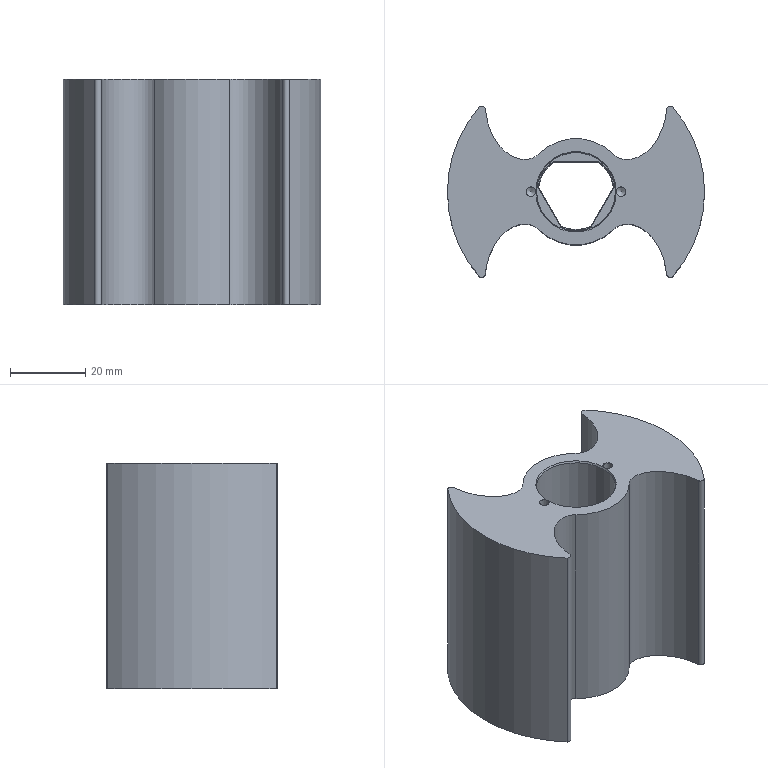NC program | NX | posted with a generic post | part box 68.489 x 45.577 x 60 mm
Lines 4138 to 5071 of 7016:
(CUTTERCOMP12 , TOOL : D12)
N8274 T12 M6
N8276 G54
N8278 G17 G0 G90 X33.59 Y-26.428 S5000 M3
N8280 G43 Z30. H12
N8282 Z1.
N8284 G94 G1 Z-1. F1250.
N8286 G41 X33.497 Y-26.392 D12
N8288 X31.512 Y-26.006
N8290 G3 X30.378 Y-26.397 R1.2
N8292 G2 X18.216 Y-22.529 R6.95
N8294 G3 X17.367 Y-18.826 R14.157
N8296 X16.037 Y-16.381 R9.956
N8298 X14.862 Y-15.174 R6.285
N8300 X13.864 Y-14.63 R3.173
N8302 G2 X-13.864 Y-14.629 R20.155
N8304 G3 X-14.862 Y-15.174 R3.211
N8306 X-16.324 Y-16.786 R6.7
N8308 X-17.543 Y-19.315 R10.577
N8310 X-18.216 Y-22.527 R14.318
N8312 G2 X-30.378 Y-26.397 R6.95
N8314 G3 X-31.512 Y-26.006 R1.2
N8316 G1 X-33.497 Y-26.392
N8318 G40
N8320 X-33.59 Y-26.428
N8322 Z1.
N8324 G0 X33.59 Z0.
N8326 G1 Z-2.
N8328 G41 X33.497 Y-26.392
N8330 X31.512 Y-26.006
N8332 G3 X30.378 Y-26.397 R1.2
N8334 G2 X18.216 Y-22.529 R6.95
N8336 G3 X17.367 Y-18.826 R14.159
N8338 X16.037 Y-16.381 R9.956
N8340 X14.862 Y-15.174 R6.285
N8342 X13.864 Y-14.63 R3.174
N8344 G2 X-13.864 Y-14.629 R20.155
N8346 G3 X-14.862 Y-15.174 R3.213
N8348 X-16.324 Y-16.786 R6.7
N8350 X-17.543 Y-19.315 R10.578
N8352 X-18.216 Y-22.527 R14.323
N8354 G2 X-30.378 Y-26.397 R6.95
N8356 G3 X-31.512 Y-26.006 R1.2
N8358 G1 X-33.497 Y-26.392
N8360 G40
N8362 X-33.59 Y-26.428
N8364 Z0.
N8366 G0 Z30.
N8368 X33.59
N8370 Z-1.
N8372 G1 Z-3.
N8374 G41 X33.497 Y-26.392
N8376 X31.512 Y-26.006
N8378 G3 X30.378 Y-26.397 R1.2
N8380 G2 X18.216 Y-22.529 R6.95
N8382 G3 X17.367 Y-18.826 R14.16
N8384 X16.037 Y-16.381 R9.955
N8386 X14.862 Y-15.174 R6.285
N8388 X13.864 Y-14.63 R3.175
N8390 G2 X-13.864 Y-14.629 R20.155
N8392 G3 X-14.862 Y-15.174 R3.214
N8394 X-16.324 Y-16.786 R6.7
N8396 X-17.543 Y-19.315 R10.579
N8398 X-18.216 Y-22.527 R14.328
N8400 G2 X-30.378 Y-26.397 R6.95
N8402 G3 X-31.512 Y-26.006 R1.2
N8404 G1 X-33.497 Y-26.392
N8406 G40
N8408 X-33.59 Y-26.428
N8410 Z-1.
N8412 G0 Z30.
N8414 X33.59
N8416 Z-2.
N8418 G1 Z-4.
N8420 G41 X33.497 Y-26.392
N8422 X31.512 Y-26.006
N8424 G3 X30.378 Y-26.397 R1.2
N8426 G2 X18.216 Y-22.529 R6.95
N8428 G3 X17.367 Y-18.826 R14.162
N8430 X16.037 Y-16.381 R9.955
N8432 X14.862 Y-15.174 R6.285
N8434 X13.864 Y-14.63 R3.175
N8436 G2 X-13.864 Y-14.629 R20.155
N8438 G3 X-14.862 Y-15.174 R3.215
N8440 X-16.039 Y-16.381 R6.439
N8442 X-17.367 Y-18.826 R10.062
N8444 X-18.216 Y-22.527 R14.147
N8446 G2 X-30.378 Y-26.397 R6.95
N8448 G3 X-31.512 Y-26.006 R1.2
N8450 G1 X-33.497 Y-26.392
N8452 G40
N8454 X-33.59 Y-26.428
N8456 Z-2.
N8458 G0 Z30.
N8460 X33.59
N8462 Z-3.
N8464 G1 Z-5.
N8466 G41 X33.497 Y-26.392
N8468 X31.512 Y-26.006
N8470 G3 X30.378 Y-26.397 R1.2
N8472 G2 X18.216 Y-22.529 R6.95
N8474 G3 X17.367 Y-18.826 R14.164
N8476 X16.037 Y-16.381 R9.955
N8478 X14.862 Y-15.174 R6.284
N8480 X13.864 Y-14.63 R3.176
N8482 G2 X-13.864 Y-14.629 R20.155
N8484 G3 X-14.862 Y-15.174 R3.216
N8486 X-16.039 Y-16.381 R6.438
N8488 X-17.367 Y-18.826 R10.06
N8490 X-18.216 Y-22.527 R14.13
N8492 G2 X-30.378 Y-26.397 R6.95
N8494 G3 X-31.512 Y-26.006 R1.2
N8496 G1 X-33.497 Y-26.392
N8498 G40
N8500 X-33.59 Y-26.428
N8502 Z-3.
N8504 G0 Z30.
N8506 X33.59
N8508 Z-4.
N8510 G1 Z-6.
N8512 G41 X33.497 Y-26.392
N8514 X31.512 Y-26.006
N8516 G3 X30.378 Y-26.397 R1.2
N8518 G2 X18.216 Y-22.529 R6.95
N8520 G3 X17.367 Y-18.826 R14.165
N8522 X16.037 Y-16.381 R9.954
N8524 X14.862 Y-15.174 R6.284
N8526 X13.864 Y-14.63 R3.177
N8528 G2 X-13.864 Y-14.629 R20.155
N8530 G3 X-14.862 Y-15.174 R3.217
N8532 X-16.039 Y-16.381 R6.436
N8534 X-17.367 Y-18.826 R10.058
N8536 X-18.216 Y-22.527 R14.133
N8538 G2 X-30.378 Y-26.397 R6.95
N8540 G3 X-31.512 Y-26.006 R1.2
N8542 G1 X-33.497 Y-26.392
N8544 G40
N8546 X-33.59 Y-26.428
N8548 Z-4.
N8550 G0 Z30.
N8552 X33.59
N8554 Z-5.
N8556 G1 Z-7.
N8558 G41 X33.497 Y-26.392
N8560 X31.512 Y-26.006
N8562 G3 X30.378 Y-26.397 R1.2
N8564 G2 X18.216 Y-22.529 R6.95
N8566 G3 X17.367 Y-18.826 R14.167
N8568 X16.037 Y-16.381 R9.954
N8570 X14.862 Y-15.174 R6.284
N8572 X13.864 Y-14.63 R3.177
N8574 G2 X-13.864 Y-14.629 R20.155
N8576 G3 X-14.862 Y-15.174 R3.218
N8578 X-16.039 Y-16.381 R6.435
N8580 X-17.367 Y-18.826 R10.057
N8582 X-18.216 Y-22.527 R14.137
N8584 G2 X-30.378 Y-26.397 R6.95
N8586 G3 X-31.512 Y-26.006 R1.2
N8588 G1 X-33.497 Y-26.392
N8590 G40
N8592 X-33.59 Y-26.428
N8594 Z-5.
N8596 G0 Z30.
N8598 X33.59
N8600 Z-6.
N8602 G1 Z-8.
N8604 G41 X33.497 Y-26.392
N8606 X31.512 Y-26.006
N8608 G3 X30.378 Y-26.397 R1.2
N8610 G2 X18.216 Y-22.529 R6.95
N8612 G3 X17.367 Y-18.826 R14.169
N8614 X16.037 Y-16.381 R9.954
N8616 X14.862 Y-15.174 R6.275
N8618 X13.864 Y-14.63 R3.178
N8620 G2 X-13.864 Y-14.629 R20.155
N8622 G3 X-14.862 Y-15.174 R3.219
N8624 X-16.038 Y-16.381 R6.434
N8626 X-17.367 Y-18.826 R10.055
N8628 X-18.216 Y-22.527 R14.141
N8630 G2 X-30.378 Y-26.397 R6.95
N8632 G3 X-31.512 Y-26.006 R1.2
N8634 G1 X-33.497 Y-26.392
N8636 G40
N8638 X-33.59 Y-26.428
N8640 Z-6.
N8642 G0 Z30.
N8644 X33.59
N8646 Z-7.
N8648 G1 Z-9.
N8650 G41 X33.497 Y-26.392
N8652 X31.512 Y-26.006
N8654 G3 X30.378 Y-26.397 R1.2
N8656 G2 X18.216 Y-22.529 R6.95
N8658 G3 X17.367 Y-18.826 R14.17
N8660 X16.037 Y-16.381 R9.953
N8662 X14.862 Y-15.174 R6.275
N8664 X13.864 Y-14.63 R3.179
N8666 G2 X-13.864 Y-14.629 R20.155
N8668 G3 X-14.862 Y-15.174 R3.22
N8670 X-16.038 Y-16.381 R6.433
N8672 X-17.367 Y-18.826 R10.054
N8674 X-18.216 Y-22.527 R14.144
N8676 G2 X-30.378 Y-26.397 R6.95
N8678 G3 X-31.512 Y-26.006 R1.2
N8680 G1 X-33.497 Y-26.392
N8682 G40
N8684 X-33.59 Y-26.428
N8686 Z-7.
N8688 G0 Z30.
N8690 X33.59
N8692 Z-8.
N8694 G1 Z-10.
N8696 G41 X33.497 Y-26.392
N8698 X31.512 Y-26.006
N8700 G3 X30.378 Y-26.397 R1.2
N8702 G2 X18.216 Y-22.529 R6.95
N8704 G3 X17.367 Y-18.826 R14.172
N8706 X16.037 Y-16.381 R9.953
N8708 X14.862 Y-15.174 R6.274
N8710 X13.864 Y-14.63 R3.179
N8712 G2 X-13.864 Y-14.629 R20.155
N8714 G3 X-14.862 Y-15.174 R3.221
N8716 X-16.038 Y-16.381 R6.432
N8718 X-17.367 Y-18.826 R10.052
N8720 X-18.216 Y-22.527 R14.148
N8722 G2 X-30.378 Y-26.397 R6.95
N8724 G3 X-31.512 Y-26.006 R1.2
N8726 G1 X-33.497 Y-26.392
N8728 G40
N8730 X-33.59 Y-26.428
N8732 Z-8.
N8734 G0 Z30.
N8736 X33.59
N8738 Z-9.
N8740 G1 Z-11.
N8742 G41 X33.497 Y-26.392
N8744 X31.512 Y-26.006
N8746 G3 X30.378 Y-26.397 R1.2
N8748 G2 X18.216 Y-22.529 R6.95
N8750 G3 X17.367 Y-18.826 R14.174
N8752 X16.037 Y-16.381 R9.953
N8754 X14.862 Y-15.174 R6.274
N8756 X13.864 Y-14.63 R3.18
N8758 G2 X-13.864 Y-14.629 R20.155
N8760 G3 X-14.862 Y-15.174 R3.222
N8762 X-16.038 Y-16.381 R6.43
N8764 X-17.367 Y-18.826 R10.051
N8766 X-18.216 Y-22.527 R14.152
N8768 G2 X-30.378 Y-26.397 R6.95
N8770 G3 X-31.512 Y-26.006 R1.2
N8772 G1 X-33.497 Y-26.392
N8774 G40
N8776 X-33.59 Y-26.428
N8778 Z-9.
N8780 G0 Z30.
N8782 X33.59
N8784 Z-10.
N8786 G1 Z-12.
N8788 G41 X33.497 Y-26.392
N8790 X31.512 Y-26.006
N8792 G3 X30.378 Y-26.397 R1.2
N8794 G2 X18.216 Y-22.529 R6.95
N8796 G3 X17.367 Y-18.826 R14.175
N8798 X16.037 Y-16.381 R9.953
N8800 X14.862 Y-15.174 R6.274
N8802 X13.864 Y-14.63 R3.18
N8804 G2 X-13.864 Y-14.629 R20.155
N8806 G3 X-14.862 Y-15.174 R3.223
N8808 X-16.038 Y-16.381 R6.429
N8810 X-17.367 Y-18.826 R10.049
N8812 X-18.216 Y-22.527 R14.155
N8814 G2 X-30.378 Y-26.397 R6.95
N8816 G3 X-31.512 Y-26.006 R1.2
N8818 G1 X-33.497 Y-26.392
N8820 G40
N8822 X-33.59 Y-26.428
N8824 Z-10.
N8826 G0 Z30.
N8828 X33.59
N8830 Z-11.
N8832 G1 Z-13.
N8834 G41 X33.497 Y-26.392
N8836 X31.512 Y-26.006
N8838 G3 X30.378 Y-26.397 R1.2
N8840 G2 X18.216 Y-22.529 R6.95
N8842 G3 X17.367 Y-18.826 R14.177
N8844 X16.037 Y-16.381 R9.952
N8846 X14.862 Y-15.174 R6.274
N8848 X13.864 Y-14.63 R3.181
N8850 G2 X-13.864 Y-14.629 R20.155
N8852 G3 X-14.862 Y-15.174 R3.224
N8854 X-16.038 Y-16.381 R6.428
N8856 X-17.367 Y-18.826 R10.048
N8858 X-18.216 Y-22.527 R14.159
N8860 G2 X-30.378 Y-26.397 R6.95
N8862 G3 X-31.512 Y-26.006 R1.2
N8864 G1 X-33.497 Y-26.392
N8866 G40
N8868 X-33.59 Y-26.428
N8870 Z-11.
N8872 G0 Z30.
N8874 X33.59
N8876 Z-12.
N8878 G1 Z-14.
N8880 G41 X33.497 Y-26.392
N8882 X31.512 Y-26.006
N8884 G3 X30.378 Y-26.397 R1.2
N8886 G2 X18.216 Y-22.529 R6.95
N8888 G3 X17.367 Y-18.826 R14.179
N8890 X16.037 Y-16.381 R9.952
N8892 X14.862 Y-15.174 R6.274
N8894 X13.864 Y-14.63 R3.182
N8896 G2 X-13.864 Y-14.629 R20.155
N8898 G3 X-14.862 Y-15.174 R3.226
N8900 X-16.038 Y-16.381 R6.427
N8902 X-17.367 Y-18.826 R10.046
N8904 X-18.216 Y-22.527 R14.163
N8906 G2 X-30.378 Y-26.397 R6.95
N8908 G3 X-31.512 Y-26.006 R1.2
N8910 G1 X-33.497 Y-26.392
N8912 G40
N8914 X-33.59 Y-26.428
N8916 Z-12.
N8918 G0 Z30.
N8920 X33.59
N8922 Z-13.
N8924 G1 Z-15.
N8926 G41 X33.497 Y-26.392
N8928 X31.512 Y-26.006
N8930 G3 X30.378 Y-26.397 R1.2
N8932 G2 X18.216 Y-22.529 R6.95
N8934 G3 X17.367 Y-18.826 R14.18
N8936 X16.037 Y-16.381 R9.952
N8938 X14.862 Y-15.174 R6.274
N8940 X13.864 Y-14.63 R3.182
N8942 G2 X-13.864 Y-14.629 R20.155
N8944 G3 X-14.862 Y-15.174 R3.227
N8946 X-16.038 Y-16.381 R6.426
N8948 X-17.367 Y-18.826 R10.045
N8950 X-18.216 Y-22.527 R14.167
N8952 G2 X-30.378 Y-26.397 R6.95
N8954 G3 X-31.512 Y-26.006 R1.2
N8956 G1 X-33.497 Y-26.392
N8958 G40
N8960 X-33.59 Y-26.428
N8962 Z-13.
N8964 G0 Z30.
N8966 X33.59
N8968 Z-14.
N8970 G1 Z-16.
N8972 G41 X33.497 Y-26.392
N8974 X31.512 Y-26.006
N8976 G3 X30.378 Y-26.397 R1.2
N8978 G2 X18.216 Y-22.529 R6.95
N8980 G3 X17.367 Y-18.826 R14.182
N8982 X16.037 Y-16.381 R9.951
N8984 X14.862 Y-15.174 R6.273
N8986 X13.864 Y-14.63 R3.183
N8988 G2 X-13.864 Y-14.629 R20.155
N8990 G3 X-14.862 Y-15.174 R3.228
N8992 X-16.324 Y-16.786 R6.71
N8994 X-17.542 Y-19.315 R10.595
N8996 X-18.216 Y-22.527 R14.393
N8998 G2 X-30.378 Y-26.397 R6.95
N9000 G3 X-31.512 Y-26.006 R1.2
N9002 G1 X-33.497 Y-26.392
N9004 G40
N9006 X-33.59 Y-26.428
N9008 Z-14.
N9010 G0 Z30.
N9012 X33.59
N9014 Z-15.
N9016 G1 Z-17.
N9018 G41 X33.497 Y-26.392
N9020 X31.512 Y-26.006
N9022 G3 X30.378 Y-26.397 R1.2
N9024 G2 X18.216 Y-22.529 R6.95
N9026 G3 X17.367 Y-18.826 R14.184
N9028 X16.037 Y-16.381 R9.951
N9030 X14.862 Y-15.174 R6.273
N9032 X13.864 Y-14.63 R3.184
N9034 G2 X-13.864 Y-14.629 R20.155
N9036 G3 X-14.862 Y-15.174 R3.229
N9038 X-16.324 Y-16.786 R6.711
N9040 X-17.542 Y-19.315 R10.597
N9042 X-18.216 Y-22.527 R14.398
N9044 G2 X-30.378 Y-26.397 R6.95
N9046 G3 X-31.512 Y-26.006 R1.2
N9048 G1 X-33.497 Y-26.392
N9050 G40
N9052 X-33.59 Y-26.428
N9054 Z-15.
N9056 G0 Z30.
N9058 X33.59
N9060 Z-16.
N9062 G1 Z-18.
N9064 G41 X33.497 Y-26.392
N9066 X31.512 Y-26.006
N9068 G3 X30.378 Y-26.397 R1.2
N9070 G2 X18.216 Y-22.529 R6.95
N9072 G3 X17.367 Y-18.826 R14.185
N9074 X16.036 Y-16.381 R9.951
N9076 X14.862 Y-15.174 R6.273
N9078 X13.864 Y-14.63 R3.184
N9080 G2 X-13.864 Y-14.629 R20.155
N9082 G3 X-14.862 Y-15.174 R3.23
N9084 X-16.324 Y-16.786 R6.712
N9086 X-17.542 Y-19.315 R10.598
N9088 X-18.216 Y-22.527 R14.403
N9090 G2 X-30.378 Y-26.397 R6.95
N9092 G3 X-31.512 Y-26.006 R1.2
N9094 G1 X-33.497 Y-26.392
N9096 G40
N9098 X-33.59 Y-26.428
N9100 Z-16.
N9102 G0 Z30.
N9104 X33.59
N9106 Z-17.
N9108 G1 Z-19.
N9110 G41 X33.497 Y-26.392
N9112 X31.512 Y-26.006
N9114 G3 X30.378 Y-26.397 R1.2
N9116 G2 X18.216 Y-22.529 R6.95
N9118 G3 X17.367 Y-18.826 R14.187
N9120 X16.036 Y-16.381 R9.95
N9122 X14.862 Y-15.174 R6.273
N9124 X13.864 Y-14.63 R3.185
N9126 G2 X-13.864 Y-14.629 R20.155
N9128 G3 X-14.862 Y-15.174 R3.231
N9130 X-16.324 Y-16.786 R6.713
N9132 X-17.542 Y-19.315 R10.599
N9134 X-18.216 Y-22.527 R14.408
N9136 G2 X-30.378 Y-26.397 R6.95
N9138 G3 X-31.512 Y-26.006 R1.2
N9140 G1 X-33.497 Y-26.392
N9142 G40
N9144 X-33.59 Y-26.428
N9146 Z-17.
N9148 G0 Z30.
N9150 X33.59
N9152 Z-18.
N9154 G1 Z-20.
N9156 G41 X33.497 Y-26.392
N9158 X31.512 Y-26.006
N9160 G3 X30.378 Y-26.397 R1.2
N9162 G2 X18.216 Y-22.529 R6.95
N9164 G3 X17.367 Y-18.826 R14.189
N9166 X16.036 Y-16.381 R9.95
N9168 X14.862 Y-15.174 R6.273
N9170 X13.864 Y-14.63 R3.186
N9172 G2 X-13.864 Y-14.629 R20.155
N9174 G3 X-14.862 Y-15.174 R3.232
N9176 X-16.324 Y-16.786 R6.714
N9178 X-17.542 Y-19.315 R10.6
N9180 X-18.216 Y-22.527 R14.413
N9182 G2 X-30.378 Y-26.397 R6.95
N9184 G3 X-31.512 Y-26.006 R1.2
N9186 G1 X-33.497 Y-26.392
N9188 G40
N9190 X-33.59 Y-26.428
N9192 Z-18.
N9194 G0 Z30.
N9196 X33.59
N9198 Z-19.
N9200 G1 Z-21.
N9202 G41 X33.497 Y-26.392
N9204 X31.512 Y-26.006
N9206 G3 X30.378 Y-26.397 R1.2
N9208 G2 X18.216 Y-22.529 R6.95
N9210 G3 X17.367 Y-18.826 R14.19
N9212 X16.036 Y-16.381 R9.95
N9214 X14.862 Y-15.174 R6.273
N9216 X13.864 Y-14.63 R3.186
N9218 G2 X-13.864 Y-14.629 R20.155
N9220 G3 X-14.862 Y-15.174 R3.233
N9222 X-16.324 Y-16.786 R6.714
N9224 X-17.542 Y-19.315 R10.602
N9226 X-18.216 Y-22.527 R14.418
N9228 G2 X-30.378 Y-26.397 R6.95
N9230 G3 X-31.512 Y-26.006 R1.2
N9232 G1 X-33.497 Y-26.392
N9234 G40
N9236 X-33.59 Y-26.428
N9238 Z-19.
N9240 G0 Z30.
N9242 X33.59
N9244 Z-20.
N9246 G1 Z-22.
N9248 G41 X33.497 Y-26.392
N9250 X31.512 Y-26.006
N9252 G3 X30.378 Y-26.397 R1.2
N9254 G2 X18.216 Y-22.529 R6.95
N9256 G3 X17.367 Y-18.826 R14.192
N9258 X16.036 Y-16.381 R9.949
N9260 X14.862 Y-15.174 R6.272
N9262 X13.864 Y-14.63 R3.187
N9264 G2 X-13.864 Y-14.629 R20.155
N9266 G3 X-14.862 Y-15.174 R3.234
N9268 X-16.324 Y-16.786 R6.715
N9270 X-17.542 Y-19.315 R10.603
N9272 X-18.216 Y-22.527 R14.424
N9274 G2 X-30.378 Y-26.397 R6.95
N9276 G3 X-31.512 Y-26.006 R1.2
N9278 G1 X-33.497 Y-26.392
N9280 G40
N9282 X-33.59 Y-26.428
N9284 Z-20.
N9286 G0 Z30.
N9288 X33.59
N9290 Z-21.
N9292 G1 Z-23.
N9294 G41 X33.497 Y-26.392
N9296 X31.512 Y-26.006
N9298 G3 X30.378 Y-26.397 R1.2
N9300 G2 X18.216 Y-22.529 R6.95
N9302 G3 X17.367 Y-18.826 R14.194
N9304 X16.036 Y-16.381 R9.949
N9306 X14.862 Y-15.174 R6.272
N9308 X13.864 Y-14.63 R3.187
N9310 G2 X-13.864 Y-14.629 R20.155
N9312 G3 X-14.862 Y-15.174 R3.235
N9314 X-16.324 Y-16.786 R6.716
N9316 X-17.542 Y-19.315 R10.604
N9318 X-18.216 Y-22.527 R14.429
N9320 G2 X-30.378 Y-26.397 R6.95
N9322 G3 X-31.512 Y-26.006 R1.2
N9324 G1 X-33.497 Y-26.392
N9326 G40
N9328 X-33.59 Y-26.428
N9330 Z-21.
N9332 G0 Z30.
N9334 X33.59
N9336 Z-22.
N9338 G1 Z-24.
N9340 G41 X33.497 Y-26.392
N9342 X31.512 Y-26.006
N9344 G3 X30.378 Y-26.397 R1.2
N9346 G2 X18.216 Y-22.529 R6.95
N9348 G3 X17.367 Y-18.826 R14.195
N9350 X16.036 Y-16.381 R9.949
N9352 X14.862 Y-15.174 R6.272
N9354 X13.864 Y-14.63 R3.188
N9356 G2 X-13.864 Y-14.629 R20.155
N9358 G3 X-14.862 Y-15.174 R3.237
N9360 X-16.324 Y-16.786 R6.717
N9362 X-17.542 Y-19.315 R10.605
N9364 X-18.216 Y-22.527 R14.434
N9366 G2 X-30.378 Y-26.397 R6.95
N9368 G3 X-31.512 Y-26.006 R1.2
N9370 G1 X-33.497 Y-26.392
N9372 G40
N9374 X-33.59 Y-26.428
N9376 Z-22.
N9378 G0 Z30.
N9380 X33.59
N9382 Z-23.
N9384 G1 Z-25.
N9386 G41 X33.497 Y-26.392
N9388 X31.512 Y-26.006
N9390 G3 X30.378 Y-26.397 R1.2
N9392 G2 X18.216 Y-22.529 R6.95
N9394 G3 X17.367 Y-18.826 R14.197
N9396 X16.036 Y-16.381 R9.948
N9398 X14.862 Y-15.174 R6.272
N9400 X13.864 Y-14.63 R3.189
N9402 G2 X-13.864 Y-14.629 R20.155
N9404 G3 X-14.862 Y-15.174 R3.238
N9406 X-16.324 Y-16.786 R6.718
N9408 X-17.542 Y-19.315 R10.607
N9410 X-18.216 Y-22.527 R14.439
N9412 G2 X-30.378 Y-26.397 R6.95
N9414 G3 X-31.512 Y-26.006 R1.2
N9416 G1 X-33.497 Y-26.392
N9418 G40
N9420 X-33.59 Y-26.428
N9422 Z-23.
N9424 G0 Z30.
N9426 X33.59
N9428 Z-24.
N9430 G1 Z-26.
N9432 G41 X33.497 Y-26.392
N9434 X31.512 Y-26.006
N9436 G3 X30.378 Y-26.397 R1.2
N9438 G2 X18.216 Y-22.529 R6.95
N9440 G3 X17.367 Y-18.826 R14.199
N9442 X16.036 Y-16.381 R9.948
N9444 X14.862 Y-15.174 R6.272
N9446 X13.864 Y-14.63 R3.189
N9448 G2 X-13.864 Y-14.629 R20.155
N9450 G3 X-14.862 Y-15.174 R3.239
N9452 X-16.324 Y-16.786 R6.718
N9454 X-17.542 Y-19.315 R10.608
N9456 X-18.216 Y-22.527 R14.444
N9458 G2 X-30.378 Y-26.397 R6.95
N9460 G3 X-31.512 Y-26.006 R1.2
N9462 G1 X-33.497 Y-26.392
N9464 G40
N9466 X-33.59 Y-26.428
N9468 Z-24.
N9470 G0 Z30.
N9472 X33.59
N9474 Z-25.
N9476 G1 Z-27.
N9478 G41 X33.497 Y-26.392
N9480 X31.512 Y-26.006
N9482 G3 X30.378 Y-26.397 R1.2
N9484 G2 X18.216 Y-22.529 R6.95
N9486 G3 X17.367 Y-18.826 R14.2
N9488 X16.036 Y-16.381 R9.948
N9490 X14.862 Y-15.174 R6.272
N9492 X13.864 Y-14.63 R3.19
N9494 G2 X-13.864 Y-14.629 R20.155
N9496 G3 X-14.862 Y-15.174 R3.24
N9498 X-16.324 Y-16.786 R6.719
N9500 X-17.542 Y-19.315 R10.609
N9502 X-18.216 Y-22.527 R14.449
N9504 G2 X-30.378 Y-26.397 R6.95
N9506 G3 X-31.512 Y-26.006 R1.2
N9508 G1 X-33.497 Y-26.392
N9510 G40
N9512 X-33.59 Y-26.428
N9514 Z-25.
N9516 G0 Z30.
N9518 X33.59
N9520 Z-26.
N9522 G1 Z-28.
N9524 G41 X33.497 Y-26.392
N9526 X31.512 Y-26.006
N9528 G3 X30.378 Y-26.397 R1.2
N9530 G2 X18.216 Y-22.529 R6.95
N9532 G3 X17.367 Y-18.826 R14.202
N9534 X16.036 Y-16.381 R9.948
N9536 X14.862 Y-15.174 R6.271
N9538 X13.864 Y-14.63 R3.191
N9540 G2 X-13.864 Y-14.629 R20.155
N9542 G3 X-14.862 Y-15.174 R3.241
N9544 X-16.324 Y-16.786 R6.72
N9546 X-17.542 Y-19.315 R10.609
N9548 X-18.216 Y-22.527 R14.454
N9550 G2 X-30.378 Y-26.397 R6.95
N9552 G3 X-31.512 Y-26.006 R1.2
N9554 G1 X-33.497 Y-26.392
N9556 G40
N9558 X-33.59 Y-26.428
N9560 Z-26.
N9562 G0 Z30.
N9564 X33.59
N9566 Z-27.
N9568 G1 Z-29.
N9570 G41 X33.497 Y-26.392
N9572 X31.512 Y-26.006
N9574 G3 X30.378 Y-26.397 R1.2
N9576 G2 X18.216 Y-22.529 R6.95
N9578 G3 X17.367 Y-18.826 R14.204
N9580 X16.036 Y-16.381 R9.947
N9582 X14.862 Y-15.174 R6.271
N9584 X13.864 Y-14.63 R3.191
N9586 G2 X-13.864 Y-14.629 R20.155
N9588 G3 X-14.862 Y-15.174 R3.242
N9590 X-16.324 Y-16.786 R6.721
N9592 X-17.542 Y-19.315 R10.609
N9594 X-18.216 Y-22.527 R14.459
N9596 G2 X-30.378 Y-26.397 R6.95
N9598 G3 X-31.512 Y-26.006 R1.2
N9600 G1 X-33.497 Y-26.392
N9602 G40
N9604 X-33.59 Y-26.428
N9606 Z-27.
N9608 G0 Z30.
N9610 X33.59
N9612 Z-28.
N9614 G1 Z-30.
N9616 G41 X33.497 Y-26.392
N9618 X31.512 Y-26.006
N9620 G3 X30.378 Y-26.397 R1.2
N9622 G2 X18.216 Y-22.529 R6.95
N9624 G3 X17.367 Y-18.826 R14.206
N9626 X16.036 Y-16.381 R9.947
N9628 X14.862 Y-15.174 R6.271
N9630 X13.864 Y-14.63 R3.192
N9632 G2 X-13.864 Y-14.629 R20.155
N9634 G3 X-14.862 Y-15.174 R3.243
N9636 X-16.324 Y-16.786 R6.722
N9638 X-17.542 Y-19.315 R10.608
N9640 X-18.216 Y-22.527 R14.464
N9642 G2 X-30.378 Y-26.397 R6.95
N9644 G3 X-31.512 Y-26.006 R1.2
N9646 G1 X-33.497 Y-26.392
N9648 G40
N9650 X-33.59 Y-26.428
N9652 Z-28.
N9654 G0 Z30.
N9656 X33.59
N9658 Z-29.
N9660 G1 Z-31.
N9662 G41 X33.497 Y-26.392
N9664 X31.512 Y-26.006
N9666 G3 X30.378 Y-26.397 R1.2
N9668 G2 X18.216 Y-22.529 R6.95
N9670 G3 X17.367 Y-18.826 R14.207
N9672 X16.036 Y-16.381 R9.947
N9674 X14.862 Y-15.174 R6.271
N9676 X13.864 Y-14.63 R3.193
N9678 G2 X-13.864 Y-14.629 R20.155
N9680 G3 X-14.862 Y-15.174 R3.244
N9682 X-16.324 Y-16.786 R6.723
N9684 X-17.541 Y-19.315 R10.608
N9686 X-18.216 Y-22.527 R14.469
N9688 G2 X-30.378 Y-26.397 R6.95
N9690 G3 X-31.512 Y-26.006 R1.2
N9692 G1 X-33.497 Y-26.392
N9694 G40
N9696 X-33.59 Y-26.428
N9698 Z-29.
N9700 G0 Z30.
N9702 X33.59
N9704 Z-30.
N9706 G1 Z-32.
N9708 G41 X33.497 Y-26.392
N9710 X31.512 Y-26.006
N9712 G3 X30.378 Y-26.397 R1.2
N9714 G2 X18.216 Y-22.529 R6.95
N9716 G3 X17.367 Y-18.826 R14.209
N9718 X16.036 Y-16.381 R9.946
N9720 X14.862 Y-15.174 R6.271
N9722 X13.864 Y-14.63 R3.193
N9724 G2 X-13.864 Y-14.629 R20.155
N9726 G3 X-14.862 Y-15.174 R3.245
N9728 X-16.324 Y-16.786 R6.723
N9730 X-17.541 Y-19.315 R10.623
N9732 X-18.216 Y-22.527 R14.474
N9734 G2 X-30.378 Y-26.397 R6.95
N9736 G3 X-31.512 Y-26.006 R1.2
N9738 G1 X-33.497 Y-26.392
N9740 G40
N9742 X-33.59 Y-26.428
N9744 Z-30.
N9746 G0 Z30.
N9748 X33.59
N9750 Z-31.
N9752 G1 Z-33.
N9754 G41 X33.497 Y-26.392
N9756 X31.512 Y-26.006
N9758 G3 X30.378 Y-26.397 R1.2
N9760 G2 X18.216 Y-22.529 R6.95
N9762 G3 X17.367 Y-18.826 R14.211
N9764 X16.036 Y-16.381 R9.946
N9766 X14.862 Y-15.175 R6.271
N9768 X13.864 Y-14.63 R3.194
N9770 G2 X-13.864 Y-14.629 R20.155
N9772 G3 X-14.862 Y-15.175 R3.246
N9774 X-16.324 Y-16.786 R6.724
N9776 X-17.541 Y-19.315 R10.623
N9778 X-18.216 Y-22.527 R14.479
N9780 G2 X-30.378 Y-26.397 R6.95
N9782 G3 X-31.512 Y-26.006 R1.2
N9784 G1 X-33.497 Y-26.392
N9786 G40
N9788 X-33.59 Y-26.428
N9790 Z-31.
N9792 G0 Z30.
N9794 X33.59
N9796 Z-32.
N9798 G1 Z-34.
N9800 G41 X33.497 Y-26.392
N9802 X31.512 Y-26.006
N9804 G3 X30.378 Y-26.397 R1.2
N9806 G2 X18.216 Y-22.529 R6.95
N9808 G3 X17.367 Y-18.826 R14.212
N9810 X16.036 Y-16.381 R9.946
N9812 X14.862 Y-15.175 R6.27
N9814 X13.864 Y-14.63 R3.194
N9816 G2 X-13.864 Y-14.629 R20.155
N9818 G3 X-14.862 Y-15.175 R3.248
N9820 X-16.324 Y-16.786 R6.725
N9822 X-17.541 Y-19.315 R10.623
N9824 X-18.216 Y-22.527 R14.484
N9826 G2 X-30.378 Y-26.397 R6.95
N9828 G3 X-31.512 Y-26.006 R1.2
N9830 G1 X-33.497 Y-26.392
N9832 G40
N9834 X-33.59 Y-26.428
N9836 Z-32.
N9838 G0 Z30.
N9840 X33.59
N9842 Z-33.
N9844 G1 Z-35.
N9846 G41 X33.497 Y-26.392
N9848 X31.512 Y-26.006
N9850 G3 X30.378 Y-26.397 R1.2
N9852 G2 X18.216 Y-22.529 R6.95
N9854 G3 X17.367 Y-18.826 R14.214
N9856 X16.036 Y-16.381 R9.945
N9858 X14.862 Y-15.175 R6.27
N9860 X13.864 Y-14.63 R3.195
N9862 G2 X-13.864 Y-14.629 R20.155
N9864 G3 X-14.862 Y-15.175 R3.249
N9866 X-16.324 Y-16.787 R6.726
N9868 X-17.541 Y-19.315 R10.622
N9870 X-18.216 Y-22.527 R14.489
N9872 G2 X-30.378 Y-26.397 R6.95
N9874 G3 X-31.512 Y-26.006 R1.2
N9876 G1 X-33.497 Y-26.392
N9878 G40
N9880 X-33.59 Y-26.428
N9882 Z-33.
N9884 G0 Z30.
N9886 X33.59
N9888 Z-34.
N9890 G1 Z-36.
N9892 G41 X33.497 Y-26.392
N9894 X31.512 Y-26.006
N9896 G3 X30.378 Y-26.397 R1.2
N9898 G2 X18.216 Y-22.529 R6.95
N9900 G3 X17.366 Y-18.826 R14.216
N9902 X16.036 Y-16.381 R9.945
N9904 X14.862 Y-15.175 R6.27
N9906 X13.864 Y-14.63 R3.196
N9908 G2 X-13.864 Y-14.629 R20.155
N9910 G3 X-14.862 Y-15.175 R3.25
N9912 X-16.324 Y-16.787 R6.727
N9914 X-17.541 Y-19.315 R10.622
N9916 X-18.216 Y-22.527 R14.494
N9918 G2 X-30.378 Y-26.397 R6.95
N9920 G3 X-31.512 Y-26.006 R1.2
N9922 G1 X-33.497 Y-26.392
N9924 G40
N9926 X-33.59 Y-26.428
N9928 Z-34.
N9930 G0 Z30.
N9932 X33.59
N9934 Z-35.
N9936 G1 Z-37.
N9938 G41 X33.497 Y-26.392
N9940 X31.512 Y-26.006
N9942 G3 X30.378 Y-26.397 R1.2
N9944 G2 X18.216 Y-22.529 R6.95
N9946 G3 X17.366 Y-18.826 R14.217
N9948 X16.036 Y-16.381 R9.945
N9950 X14.862 Y-15.175 R6.27
N9952 X13.864 Y-14.63 R3.196
N9954 G2 X-13.864 Y-14.629 R20.155
N9956 G3 X-14.862 Y-15.175 R3.251
N9958 X-16.324 Y-16.787 R6.727
N9960 X-17.541 Y-19.315 R10.621
N9962 X-18.216 Y-22.527 R14.5
N9964 G2 X-30.378 Y-26.397 R6.95
N9966 G3 X-31.512 Y-26.006 R1.2
N9968 G1 X-33.497 Y-26.392
N9970 G40
N9972 X-33.59 Y-26.428
N9974 Z-35.
N9976 G0 Z30.
N9978 X33.59
N9980 Z-36.
N9982 G1 Z-38.
N9984 G41 X33.497 Y-26.392
N9986 X31.512 Y-26.006
N9988 G3 X30.378 Y-26.397 R1.2
N9990 G2 X18.216 Y-22.529 R6.95
N9992 G3 X17.366 Y-18.826 R14.219
N9994 X16.036 Y-16.381 R9.944
N9996 X14.862 Y-15.175 R6.27
N9998 X13.864 Y-14.63 R3.197
N10000 G2 X-13.864 Y-14.629 R20.155
N10002 G3 X-14.862 Y-15.175 R3.252
N10004 X-16.324 Y-16.787 R6.728
N10006 X-17.541 Y-19.315 R10.621
N10008 X-18.216 Y-22.527 R14.505
N10010 G2 X-30.378 Y-26.397 R6.95
N10012 G3 X-31.512 Y-26.006 R1.2
N10014 G1 X-33.497 Y-26.392
N10016 G40
N10018 X-33.59 Y-26.428
N10020 Z-36.
N10022 G0 Z30.
N10024 X33.59
N10026 Z-37.
N10028 G1 Z-39.
N10030 G41 X33.497 Y-26.392
N10032 X31.512 Y-26.006
N10034 G3 X30.378 Y-26.397 R1.2
N10036 G2 X18.216 Y-22.529 R6.95
N10038 G3 X17.366 Y-18.826 R14.221
N10040 X16.036 Y-16.381 R9.944
N10042 X14.862 Y-15.175 R6.27
N10044 X13.864 Y-14.63 R3.198
N10046 G2 X-13.864 Y-14.629 R20.155
N10048 G3 X-14.862 Y-15.175 R3.253
N10050 X-16.324 Y-16.787 R6.729
N10052 X-17.541 Y-19.315 R10.621
N10054 X-18.216 Y-22.527 R14.51
N10056 G2 X-30.378 Y-26.397 R6.95
N10058 G3 X-31.512 Y-26.006 R1.2
N10060 G1 X-33.497 Y-26.392
N10062 G40
N10064 X-33.59 Y-26.428
N10066 Z-37.
N10068 G0 Z30.
N10070 X33.59
N10072 Z-38.
N10074 G1 Z-40.
N10076 G41 X33.497 Y-26.392
N10078 X31.512 Y-26.006
N10080 G3 X30.378 Y-26.397 R1.2
N10082 G2 X18.216 Y-22.529 R6.95
N10084 G3 X17.366 Y-18.826 R14.222
N10086 X16.036 Y-16.381 R9.944
N10088 X14.862 Y-15.175 R6.269
N10090 X13.864 Y-14.63 R3.198
N10092 G2 X-13.864 Y-14.629 R20.155
N10094 G3 X-14.862 Y-15.175 R3.254
N10096 X-16.324 Y-16.787 R6.73
N10098 X-17.541 Y-19.315 R10.623
N10100 X-18.216 Y-22.527 R14.515
N10102 G2 X-30.378 Y-26.397 R6.95
N10104 G3 X-31.512 Y-26.006 R1.2
N10106 G1 X-33.497 Y-26.392
N10108 G40
N10110 X-33.59 Y-26.428
N10112 Z-38.
N10114 G0 Z30.
N10116 X33.59
N10118 Z-39.
N10120 G1 Z-41.
N10122 G41 X33.497 Y-26.392
N10124 X31.512 Y-26.006
N10126 G3 X30.378 Y-26.397 R1.2
N10128 G2 X18.216 Y-22.529 R6.95
N10130 G3 X17.366 Y-18.826 R14.224
N10132 X16.036 Y-16.381 R9.943
N10134 X14.862 Y-15.175 R6.269